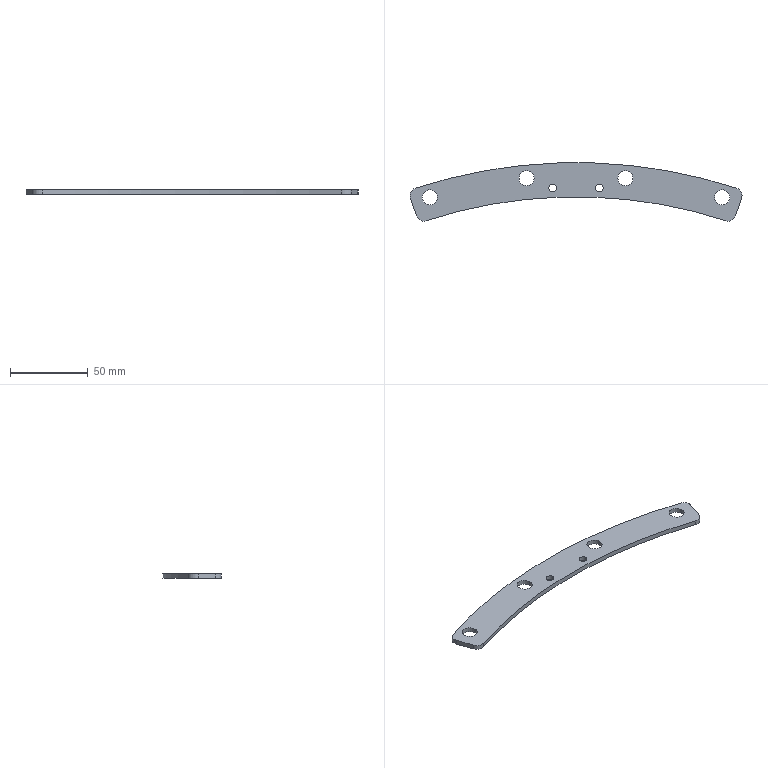Part | 1 solid | 23 faces | box 213.441 x 37.571 x 3 mm | volume 12982 mm3 | cylinder 19 | plane 4 | commonest cylinder face diameters 9.7 x8 10 x5 5 x4 620 x1 664 x1
STEP:
#1=CARTESIAN_POINT('',(-17.5,315.7,-3.));
#2=VERTEX_POINT('',#1);
#3=CARTESIAN_POINT('',(-12.5,315.7,-3.));
#4=VERTEX_POINT('',#3);
#5=CARTESIAN_POINT('',(-15.,315.7,-3.));
#6=DIRECTION('',(0.,0.,1.));
#7=DIRECTION('',(1.,0.,0.));
#8=AXIS2_PLACEMENT_3D('',#5,#6,#7);
#9=CIRCLE('',#8,2.5);
#10=EDGE_CURVE('',#2,#4,#9,.T.);
#11=ORIENTED_EDGE('',*,*,#10,.F.);
#12=CARTESIAN_POINT('',(-17.5,315.7,0.));
#13=VERTEX_POINT('',#12);
#14=CARTESIAN_POINT('',(-17.5,315.7,0.));
#15=DIRECTION('',(0.,0.,1.));
#16=VECTOR('',#15,1000.);
#17=LINE('',#14,#16);
#18=EDGE_CURVE('',#2,#13,#17,.T.);
#19=ORIENTED_EDGE('',*,*,#18,.T.);
#20=CARTESIAN_POINT('',(-12.5,315.7,0.));
#21=VERTEX_POINT('',#20);
#22=CARTESIAN_POINT('',(-15.,315.7,0.));
#23=DIRECTION('',(0.,0.,1.));
#24=DIRECTION('',(1.,0.,0.));
#25=AXIS2_PLACEMENT_3D('',#22,#23,#24);
#26=CIRCLE('',#25,2.5);
#27=EDGE_CURVE('',#13,#21,#26,.T.);
#28=ORIENTED_EDGE('',*,*,#27,.T.);
#29=CARTESIAN_POINT('',(-12.5,315.7,0.));
#30=DIRECTION('',(0.,0.,1.));
#31=VECTOR('',#30,1000.);
#32=LINE('',#29,#31);
#33=EDGE_CURVE('',#4,#21,#32,.T.);
#34=ORIENTED_EDGE('',*,*,#33,.F.);
#35=EDGE_LOOP('',(#11,#19,#28,#34));
#36=FACE_OUTER_BOUND('',#35,.T.);
#37=CARTESIAN_POINT('',(-15.,315.7,0.));
#38=DIRECTION('',(0.,0.,1.));
#39=DIRECTION('',(1.,0.,0.));
#40=AXIS2_PLACEMENT_3D('',#37,#38,#39);
#41=CYLINDRICAL_SURFACE('',#40,2.5);
#42=ADVANCED_FACE('',(#36),#41,.F.);
#43=CARTESIAN_POINT('',(12.5,315.7,-3.));
#44=VERTEX_POINT('',#43);
#45=CARTESIAN_POINT('',(17.5,315.7,-3.));
#46=VERTEX_POINT('',#45);
#47=CARTESIAN_POINT('',(15.,315.7,-3.));
#48=DIRECTION('',(0.,0.,1.));
#49=DIRECTION('',(1.,0.,0.));
#50=AXIS2_PLACEMENT_3D('',#47,#48,#49);
#51=CIRCLE('',#50,2.5);
#52=EDGE_CURVE('',#44,#46,#51,.T.);
#53=ORIENTED_EDGE('',*,*,#52,.F.);
#54=CARTESIAN_POINT('',(12.5,315.7,0.));
#55=VERTEX_POINT('',#54);
#56=CARTESIAN_POINT('',(12.5,315.7,0.));
#57=DIRECTION('',(0.,0.,1.));
#58=VECTOR('',#57,1000.);
#59=LINE('',#56,#58);
#60=EDGE_CURVE('',#44,#55,#59,.T.);
#61=ORIENTED_EDGE('',*,*,#60,.T.);
#62=CARTESIAN_POINT('',(17.5,315.7,0.));
#63=VERTEX_POINT('',#62);
#64=CARTESIAN_POINT('',(15.,315.7,0.));
#65=DIRECTION('',(0.,0.,1.));
#66=DIRECTION('',(1.,0.,0.));
#67=AXIS2_PLACEMENT_3D('',#64,#65,#66);
#68=CIRCLE('',#67,2.5);
#69=EDGE_CURVE('',#55,#63,#68,.T.);
#70=ORIENTED_EDGE('',*,*,#69,.T.);
#71=CARTESIAN_POINT('',(17.5,315.7,0.));
#72=DIRECTION('',(0.,0.,1.));
#73=VECTOR('',#72,1000.);
#74=LINE('',#71,#73);
#75=EDGE_CURVE('',#46,#63,#74,.T.);
#76=ORIENTED_EDGE('',*,*,#75,.F.);
#77=EDGE_LOOP('',(#53,#61,#70,#76));
#78=FACE_OUTER_BOUND('',#77,.T.);
#79=CARTESIAN_POINT('',(15.,315.7,0.));
#80=DIRECTION('',(0.,0.,1.));
#81=DIRECTION('',(1.,0.,0.));
#82=AXIS2_PLACEMENT_3D('',#79,#80,#81);
#83=CYLINDRICAL_SURFACE('',#82,2.5);
#84=ADVANCED_FACE('',(#78),#83,.F.);
#85=CARTESIAN_POINT('',(-89.15,309.625,-3.));
#86=VERTEX_POINT('',#85);
#87=CARTESIAN_POINT('',(-98.85,309.625,-3.));
#88=VERTEX_POINT('',#87);
#89=CARTESIAN_POINT('',(-94.,309.625,-3.));
#90=DIRECTION('',(0.,0.,-1.));
#91=DIRECTION('',(-1.,0.,0.));
#92=AXIS2_PLACEMENT_3D('',#89,#90,#91);
#93=CIRCLE('',#92,4.85);
#94=EDGE_CURVE('',#86,#88,#93,.T.);
#95=ORIENTED_EDGE('',*,*,#94,.T.);
#96=CARTESIAN_POINT('',(-98.85,309.625,0.));
#97=VERTEX_POINT('',#96);
#98=CARTESIAN_POINT('',(-98.85,309.625,-10.));
#99=DIRECTION('',(0.,0.,1.));
#100=VECTOR('',#99,1000.);
#101=LINE('',#98,#100);
#102=EDGE_CURVE('',#88,#97,#101,.T.);
#103=ORIENTED_EDGE('',*,*,#102,.T.);
#104=CARTESIAN_POINT('',(-89.15,309.625,0.));
#105=VERTEX_POINT('',#104);
#106=CARTESIAN_POINT('',(-94.,309.625,0.));
#107=DIRECTION('',(0.,0.,1.));
#108=DIRECTION('',(-1.,0.,0.));
#109=AXIS2_PLACEMENT_3D('',#106,#107,#108);
#110=CIRCLE('',#109,4.85);
#111=EDGE_CURVE('',#97,#105,#110,.T.);
#112=ORIENTED_EDGE('',*,*,#111,.T.);
#113=CARTESIAN_POINT('',(-89.15,309.625,-10.));
#114=DIRECTION('',(0.,0.,1.));
#115=VECTOR('',#114,1000.);
#116=LINE('',#113,#115);
#117=EDGE_CURVE('',#86,#105,#116,.T.);
#118=ORIENTED_EDGE('',*,*,#117,.F.);
#119=EDGE_LOOP('',(#95,#103,#112,#118));
#120=FACE_OUTER_BOUND('',#119,.T.);
#121=CARTESIAN_POINT('',(-94.,309.625,-10.));
#122=DIRECTION('',(0.,0.,1.));
#123=DIRECTION('',(1.,0.,0.));
#124=AXIS2_PLACEMENT_3D('',#121,#122,#123);
#125=CYLINDRICAL_SURFACE('',#124,4.85);
#126=ADVANCED_FACE('',(#120),#125,.F.);
#127=CARTESIAN_POINT('',(98.85,309.625,-3.));
#128=VERTEX_POINT('',#127);
#129=CARTESIAN_POINT('',(89.15,309.625,-3.));
#130=VERTEX_POINT('',#129);
#131=CARTESIAN_POINT('',(94.,309.625,-3.));
#132=DIRECTION('',(0.,0.,-1.));
#133=DIRECTION('',(-1.,0.,0.));
#134=AXIS2_PLACEMENT_3D('',#131,#132,#133);
#135=CIRCLE('',#134,4.85);
#136=EDGE_CURVE('',#128,#130,#135,.T.);
#137=ORIENTED_EDGE('',*,*,#136,.T.);
#138=CARTESIAN_POINT('',(89.15,309.625,0.));
#139=VERTEX_POINT('',#138);
#140=CARTESIAN_POINT('',(89.15,309.625,-10.));
#141=DIRECTION('',(0.,0.,1.));
#142=VECTOR('',#141,1000.);
#143=LINE('',#140,#142);
#144=EDGE_CURVE('',#130,#139,#143,.T.);
#145=ORIENTED_EDGE('',*,*,#144,.T.);
#146=CARTESIAN_POINT('',(98.85,309.625,0.));
#147=VERTEX_POINT('',#146);
#148=CARTESIAN_POINT('',(94.,309.625,0.));
#149=DIRECTION('',(0.,0.,1.));
#150=DIRECTION('',(1.,0.,0.));
#151=AXIS2_PLACEMENT_3D('',#148,#149,#150);
#152=CIRCLE('',#151,4.85);
#153=EDGE_CURVE('',#139,#147,#152,.T.);
#154=ORIENTED_EDGE('',*,*,#153,.T.);
#155=CARTESIAN_POINT('',(98.85,309.625,-10.));
#156=DIRECTION('',(0.,0.,1.));
#157=VECTOR('',#156,1000.);
#158=LINE('',#155,#157);
#159=EDGE_CURVE('',#128,#147,#158,.T.);
#160=ORIENTED_EDGE('',*,*,#159,.F.);
#161=EDGE_LOOP('',(#137,#145,#154,#160));
#162=FACE_OUTER_BOUND('',#161,.T.);
#163=CARTESIAN_POINT('',(94.,309.625,-10.));
#164=DIRECTION('',(0.,0.,1.));
#165=DIRECTION('',(1.,0.,0.));
#166=AXIS2_PLACEMENT_3D('',#163,#164,#165);
#167=CYLINDRICAL_SURFACE('',#166,4.85);
#168=ADVANCED_FACE('',(#162),#167,.F.);
#169=CARTESIAN_POINT('',(36.6,322.001,-3.));
#170=VERTEX_POINT('',#169);
#171=CARTESIAN_POINT('',(26.9,322.001,-3.));
#172=VERTEX_POINT('',#171);
#173=CARTESIAN_POINT('',(31.75,322.001,-3.));
#174=DIRECTION('',(0.,0.,-1.));
#175=DIRECTION('',(-1.,0.,0.));
#176=AXIS2_PLACEMENT_3D('',#173,#174,#175);
#177=CIRCLE('',#176,4.85);
#178=EDGE_CURVE('',#170,#172,#177,.T.);
#179=ORIENTED_EDGE('',*,*,#178,.T.);
#180=CARTESIAN_POINT('',(26.9,322.001,0.));
#181=VERTEX_POINT('',#180);
#182=CARTESIAN_POINT('',(26.9,322.001,-10.));
#183=DIRECTION('',(0.,0.,1.));
#184=VECTOR('',#183,1000.);
#185=LINE('',#182,#184);
#186=EDGE_CURVE('',#172,#181,#185,.T.);
#187=ORIENTED_EDGE('',*,*,#186,.T.);
#188=CARTESIAN_POINT('',(36.6,322.001,0.));
#189=VERTEX_POINT('',#188);
#190=CARTESIAN_POINT('',(31.75,322.001,0.));
#191=DIRECTION('',(0.,0.,1.));
#192=DIRECTION('',(1.,0.,0.));
#193=AXIS2_PLACEMENT_3D('',#190,#191,#192);
#194=CIRCLE('',#193,4.85);
#195=EDGE_CURVE('',#181,#189,#194,.T.);
#196=ORIENTED_EDGE('',*,*,#195,.T.);
#197=CARTESIAN_POINT('',(36.6,322.001,-10.));
#198=DIRECTION('',(0.,0.,1.));
#199=VECTOR('',#198,1000.);
#200=LINE('',#197,#199);
#201=EDGE_CURVE('',#170,#189,#200,.T.);
#202=ORIENTED_EDGE('',*,*,#201,.F.);
#203=EDGE_LOOP('',(#179,#187,#196,#202));
#204=FACE_OUTER_BOUND('',#203,.T.);
#205=CARTESIAN_POINT('',(31.75,322.001,-10.));
#206=DIRECTION('',(0.,0.,1.));
#207=DIRECTION('',(1.,0.,0.));
#208=AXIS2_PLACEMENT_3D('',#205,#206,#207);
#209=CYLINDRICAL_SURFACE('',#208,4.85);
#210=ADVANCED_FACE('',(#204),#209,.F.);
#211=CARTESIAN_POINT('',(-26.9,322.001,-3.));
#212=VERTEX_POINT('',#211);
#213=CARTESIAN_POINT('',(-36.6,322.001,-3.));
#214=VERTEX_POINT('',#213);
#215=CARTESIAN_POINT('',(-31.75,322.001,-3.));
#216=DIRECTION('',(0.,0.,-1.));
#217=DIRECTION('',(-1.,0.,0.));
#218=AXIS2_PLACEMENT_3D('',#215,#216,#217);
#219=CIRCLE('',#218,4.85);
#220=EDGE_CURVE('',#212,#214,#219,.T.);
#221=ORIENTED_EDGE('',*,*,#220,.T.);
#222=CARTESIAN_POINT('',(-36.6,322.001,0.));
#223=VERTEX_POINT('',#222);
#224=CARTESIAN_POINT('',(-36.6,322.001,-10.));
#225=DIRECTION('',(0.,0.,1.));
#226=VECTOR('',#225,1000.);
#227=LINE('',#224,#226);
#228=EDGE_CURVE('',#214,#223,#227,.T.);
#229=ORIENTED_EDGE('',*,*,#228,.T.);
#230=CARTESIAN_POINT('',(-26.9,322.001,0.));
#231=VERTEX_POINT('',#230);
#232=CARTESIAN_POINT('',(-31.75,322.001,0.));
#233=DIRECTION('',(0.,0.,1.));
#234=DIRECTION('',(-1.,0.,0.));
#235=AXIS2_PLACEMENT_3D('',#232,#233,#234);
#236=CIRCLE('',#235,4.85);
#237=EDGE_CURVE('',#223,#231,#236,.T.);
#238=ORIENTED_EDGE('',*,*,#237,.T.);
#239=CARTESIAN_POINT('',(-26.9,322.001,-10.));
#240=DIRECTION('',(0.,0.,1.));
#241=VECTOR('',#240,1000.);
#242=LINE('',#239,#241);
#243=EDGE_CURVE('',#212,#231,#242,.T.);
#244=ORIENTED_EDGE('',*,*,#243,.F.);
#245=EDGE_LOOP('',(#221,#229,#238,#244));
#246=FACE_OUTER_BOUND('',#245,.T.);
#247=CARTESIAN_POINT('',(-31.75,322.001,-10.));
#248=DIRECTION('',(0.,0.,1.));
#249=DIRECTION('',(1.,0.,0.));
#250=AXIS2_PLACEMENT_3D('',#247,#248,#249);
#251=CYLINDRICAL_SURFACE('',#250,4.85);
#252=ADVANCED_FACE('',(#246),#251,.F.);
#253=CARTESIAN_POINT('',(106.721,310.776,-3.));
#254=VERTEX_POINT('',#253);
#255=CARTESIAN_POINT('',(106.448,309.148,-3.));
#256=VERTEX_POINT('',#255);
#257=CARTESIAN_POINT('',(101.721,310.776,-3.));
#258=DIRECTION('',(0.,0.,-1.));
#259=DIRECTION('',(-1.,0.,0.));
#260=AXIS2_PLACEMENT_3D('',#257,#258,#259);
#261=CIRCLE('',#260,5.);
#262=EDGE_CURVE('',#254,#256,#261,.T.);
#263=ORIENTED_EDGE('',*,*,#262,.F.);
#264=CARTESIAN_POINT('',(106.721,310.776,0.));
#265=VERTEX_POINT('',#264);
#266=CARTESIAN_POINT('',(106.721,310.776,-3.));
#267=DIRECTION('',(0.,0.,1.));
#268=VECTOR('',#267,1000.);
#269=LINE('',#266,#268);
#270=EDGE_CURVE('',#254,#265,#269,.T.);
#271=ORIENTED_EDGE('',*,*,#270,.T.);
#272=CARTESIAN_POINT('',(106.448,309.148,0.));
#273=VERTEX_POINT('',#272);
#274=CARTESIAN_POINT('',(101.721,310.776,0.));
#275=DIRECTION('',(0.,0.,1.));
#276=DIRECTION('',(-1.,0.,0.));
#277=AXIS2_PLACEMENT_3D('',#274,#275,#276);
#278=CIRCLE('',#277,5.);
#279=EDGE_CURVE('',#273,#265,#278,.T.);
#280=ORIENTED_EDGE('',*,*,#279,.F.);
#281=CARTESIAN_POINT('',(106.448,309.148,-3.));
#282=DIRECTION('',(0.,0.,1.));
#283=VECTOR('',#282,1000.);
#284=LINE('',#281,#283);
#285=EDGE_CURVE('',#256,#273,#284,.T.);
#286=ORIENTED_EDGE('',*,*,#285,.F.);
#287=EDGE_LOOP('',(#263,#271,#280,#286));
#288=FACE_OUTER_BOUND('',#287,.T.);
#289=CARTESIAN_POINT('',(101.721,310.776,-3.));
#290=DIRECTION('',(0.,0.,1.));
#291=DIRECTION('',(1.,0.,0.));
#292=AXIS2_PLACEMENT_3D('',#289,#290,#291);
#293=CYLINDRICAL_SURFACE('',#292,5.);
#294=ADVANCED_FACE('',(#288),#293,.T.);
#295=CARTESIAN_POINT('',(-96.261,294.676,-3.));
#296=VERTEX_POINT('',#295);
#297=CARTESIAN_POINT('',(96.261,294.676,-3.));
#298=VERTEX_POINT('',#297);
#299=CARTESIAN_POINT('',(0.,0.,-3.));
#300=DIRECTION('',(0.,0.,-1.));
#301=DIRECTION('',(-1.,0.,0.));
#302=AXIS2_PLACEMENT_3D('',#299,#300,#301);
#303=CIRCLE('',#302,310.);
#304=EDGE_CURVE('',#296,#298,#303,.T.);
#305=ORIENTED_EDGE('',*,*,#304,.T.);
#306=CARTESIAN_POINT('',(96.261,294.676,0.));
#307=VERTEX_POINT('',#306);
#308=CARTESIAN_POINT('',(96.261,294.676,-3.));
#309=DIRECTION('',(0.,0.,1.));
#310=VECTOR('',#309,1000.);
#311=LINE('',#308,#310);
#312=EDGE_CURVE('',#298,#307,#311,.T.);
#313=ORIENTED_EDGE('',*,*,#312,.T.);
#314=CARTESIAN_POINT('',(-96.261,294.676,0.));
#315=VERTEX_POINT('',#314);
#316=CARTESIAN_POINT('',(0.,0.,0.));
#317=DIRECTION('',(0.,0.,-1.));
#318=DIRECTION('',(-1.,0.,0.));
#319=AXIS2_PLACEMENT_3D('',#316,#317,#318);
#320=CIRCLE('',#319,310.);
#321=EDGE_CURVE('',#315,#307,#320,.T.);
#322=ORIENTED_EDGE('',*,*,#321,.F.);
#323=CARTESIAN_POINT('',(-96.261,294.676,-3.));
#324=DIRECTION('',(0.,0.,-1.));
#325=VECTOR('',#324,1000.);
#326=LINE('',#323,#325);
#327=EDGE_CURVE('',#315,#296,#326,.T.);
#328=ORIENTED_EDGE('',*,*,#327,.T.);
#329=EDGE_LOOP('',(#305,#313,#322,#328));
#330=FACE_OUTER_BOUND('',#329,.T.);
#331=CARTESIAN_POINT('',(0.,0.,-3.));
#332=DIRECTION('',(0.,0.,1.));
#333=DIRECTION('',(1.,0.,0.));
#334=AXIS2_PLACEMENT_3D('',#331,#332,#333);
#335=CYLINDRICAL_SURFACE('',#334,310.);
#336=ADVANCED_FACE('',(#330),#335,.F.);
#337=CARTESIAN_POINT('',(-106.448,309.148,-3.));
#338=VERTEX_POINT('',#337);
#339=CARTESIAN_POINT('',(-102.541,297.801,-3.));
#340=VERTEX_POINT('',#339);
#341=CARTESIAN_POINT('',(-100.926,293.111,-3.));
#342=DIRECTION('',(0.3256,-0.9455,0.));
#343=VECTOR('',#342,1000.);
#344=LINE('',#341,#343);
#345=EDGE_CURVE('',#338,#340,#344,.T.);
#346=ORIENTED_EDGE('',*,*,#345,.T.);
#347=CARTESIAN_POINT('',(-102.541,297.801,0.));
#348=VERTEX_POINT('',#347);
#349=CARTESIAN_POINT('',(-102.541,297.801,-3.));
#350=DIRECTION('',(0.,0.,1.));
#351=VECTOR('',#350,1000.);
#352=LINE('',#349,#351);
#353=EDGE_CURVE('',#340,#348,#352,.T.);
#354=ORIENTED_EDGE('',*,*,#353,.T.);
#355=CARTESIAN_POINT('',(-106.448,309.148,0.));
#356=VERTEX_POINT('',#355);
#357=CARTESIAN_POINT('',(-100.926,293.111,0.));
#358=DIRECTION('',(0.3256,-0.9455,0.));
#359=VECTOR('',#358,1000.);
#360=LINE('',#357,#359);
#361=EDGE_CURVE('',#356,#348,#360,.T.);
#362=ORIENTED_EDGE('',*,*,#361,.F.);
#363=CARTESIAN_POINT('',(-106.448,309.148,-3.));
#364=DIRECTION('',(0.,0.,-1.));
#365=VECTOR('',#364,1000.);
#366=LINE('',#363,#365);
#367=EDGE_CURVE('',#356,#338,#366,.T.);
#368=ORIENTED_EDGE('',*,*,#367,.T.);
#369=EDGE_LOOP('',(#346,#354,#362,#368));
#370=FACE_OUTER_BOUND('',#369,.T.);
#371=CARTESIAN_POINT('',(-100.926,293.111,-3.));
#372=DIRECTION('',(-0.9455,-0.3256,0.));
#373=DIRECTION('',(0.3256,-0.9455,0.));
#374=AXIS2_PLACEMENT_3D('',#371,#372,#373);
#375=PLANE('',#374);
#376=ADVANCED_FACE('',(#370),#375,.T.);
#377=CARTESIAN_POINT('',(103.276,315.528,0.));
#378=VERTEX_POINT('',#377);
#379=CARTESIAN_POINT('',(-103.276,315.528,0.));
#380=VERTEX_POINT('',#379);
#381=CARTESIAN_POINT('',(0.,0.,0.));
#382=DIRECTION('',(0.,0.,1.));
#383=DIRECTION('',(-1.,0.,0.));
#384=AXIS2_PLACEMENT_3D('',#381,#382,#383);
#385=CIRCLE('',#384,332.);
#386=EDGE_CURVE('',#378,#380,#385,.T.);
#387=ORIENTED_EDGE('',*,*,#386,.F.);
#388=CARTESIAN_POINT('',(103.276,315.528,-3.));
#389=VERTEX_POINT('',#388);
#390=CARTESIAN_POINT('',(103.276,315.528,-3.));
#391=DIRECTION('',(0.,0.,-1.));
#392=VECTOR('',#391,1000.);
#393=LINE('',#390,#392);
#394=EDGE_CURVE('',#378,#389,#393,.T.);
#395=ORIENTED_EDGE('',*,*,#394,.T.);
#396=CARTESIAN_POINT('',(-103.276,315.528,-3.));
#397=VERTEX_POINT('',#396);
#398=CARTESIAN_POINT('',(0.,0.,-3.));
#399=DIRECTION('',(0.,0.,1.));
#400=DIRECTION('',(-1.,0.,0.));
#401=AXIS2_PLACEMENT_3D('',#398,#399,#400);
#402=CIRCLE('',#401,332.);
#403=EDGE_CURVE('',#389,#397,#402,.T.);
#404=ORIENTED_EDGE('',*,*,#403,.T.);
#405=CARTESIAN_POINT('',(-103.276,315.528,-3.));
#406=DIRECTION('',(0.,0.,1.));
#407=VECTOR('',#406,1000.);
#408=LINE('',#405,#407);
#409=EDGE_CURVE('',#397,#380,#408,.T.);
#410=ORIENTED_EDGE('',*,*,#409,.T.);
#411=EDGE_LOOP('',(#387,#395,#404,#410));
#412=FACE_OUTER_BOUND('',#411,.T.);
#413=CARTESIAN_POINT('',(0.,0.,-3.));
#414=DIRECTION('',(0.,0.,1.));
#415=DIRECTION('',(1.,0.,0.));
#416=AXIS2_PLACEMENT_3D('',#413,#414,#415);
#417=CYLINDRICAL_SURFACE('',#416,332.);
#418=ADVANCED_FACE('',(#412),#417,.T.);
#419=CARTESIAN_POINT('',(102.541,297.801,0.));
#420=VERTEX_POINT('',#419);
#421=CARTESIAN_POINT('',(100.926,293.111,0.));
#422=DIRECTION('',(0.3256,0.9455,0.));
#423=VECTOR('',#422,1000.);
#424=LINE('',#421,#423);
#425=EDGE_CURVE('',#420,#273,#424,.T.);
#426=ORIENTED_EDGE('',*,*,#425,.F.);
#427=CARTESIAN_POINT('',(102.541,297.801,-3.));
#428=VERTEX_POINT('',#427);
#429=CARTESIAN_POINT('',(102.541,297.801,-3.));
#430=DIRECTION('',(0.,0.,-1.));
#431=VECTOR('',#430,1000.);
#432=LINE('',#429,#431);
#433=EDGE_CURVE('',#420,#428,#432,.T.);
#434=ORIENTED_EDGE('',*,*,#433,.T.);
#435=CARTESIAN_POINT('',(100.926,293.111,-3.));
#436=DIRECTION('',(0.3256,0.9455,0.));
#437=VECTOR('',#436,1000.);
#438=LINE('',#435,#437);
#439=EDGE_CURVE('',#428,#256,#438,.T.);
#440=ORIENTED_EDGE('',*,*,#439,.T.);
#441=ORIENTED_EDGE('',*,*,#285,.T.);
#442=EDGE_LOOP('',(#426,#434,#440,#441));
#443=FACE_OUTER_BOUND('',#442,.T.);
#444=CARTESIAN_POINT('',(100.926,293.111,-3.));
#445=DIRECTION('',(0.9455,-0.3256,0.));
#446=DIRECTION('',(0.3256,0.9455,0.));
#447=AXIS2_PLACEMENT_3D('',#444,#445,#446);
#448=PLANE('',#447);
#449=ADVANCED_FACE('',(#443),#448,.T.);
#450=CARTESIAN_POINT('',(-15.,315.7,-3.));
#451=DIRECTION('',(0.,0.,1.));
#452=DIRECTION('',(1.,0.,0.));
#453=AXIS2_PLACEMENT_3D('',#450,#451,#452);
#454=CIRCLE('',#453,2.5);
#455=EDGE_CURVE('',#4,#2,#454,.T.);
#456=ORIENTED_EDGE('',*,*,#455,.T.);
#457=ORIENTED_EDGE('',*,*,#10,.T.);
#458=EDGE_LOOP('',(#456,#457));
#459=FACE_BOUND('',#458,.T.);
#460=CARTESIAN_POINT('',(15.,315.7,-3.));
#461=DIRECTION('',(0.,0.,1.));
#462=DIRECTION('',(1.,0.,0.));
#463=AXIS2_PLACEMENT_3D('',#460,#461,#462);
#464=CIRCLE('',#463,2.5);
#465=EDGE_CURVE('',#46,#44,#464,.T.);
#466=ORIENTED_EDGE('',*,*,#465,.T.);
#467=ORIENTED_EDGE('',*,*,#52,.T.);
#468=EDGE_LOOP('',(#466,#467));
#469=FACE_BOUND('',#468,.T.);
#470=ORIENTED_EDGE('',*,*,#94,.F.);
#471=CARTESIAN_POINT('',(-94.,309.625,-3.));
#472=DIRECTION('',(0.,0.,-1.));
#473=DIRECTION('',(-1.,0.,0.));
#474=AXIS2_PLACEMENT_3D('',#471,#472,#473);
#475=CIRCLE('',#474,4.85);
#476=EDGE_CURVE('',#88,#86,#475,.T.);
#477=ORIENTED_EDGE('',*,*,#476,.F.);
#478=EDGE_LOOP('',(#470,#477));
#479=FACE_BOUND('',#478,.T.);
#480=ORIENTED_EDGE('',*,*,#136,.F.);
#481=CARTESIAN_POINT('',(94.,309.625,-3.));
#482=DIRECTION('',(0.,0.,-1.));
#483=DIRECTION('',(-1.,0.,0.));
#484=AXIS2_PLACEMENT_3D('',#481,#482,#483);
#485=CIRCLE('',#484,4.85);
#486=EDGE_CURVE('',#130,#128,#485,.T.);
#487=ORIENTED_EDGE('',*,*,#486,.F.);
#488=EDGE_LOOP('',(#480,#487));
#489=FACE_BOUND('',#488,.T.);
#490=ORIENTED_EDGE('',*,*,#178,.F.);
#491=CARTESIAN_POINT('',(31.75,322.001,-3.));
#492=DIRECTION('',(0.,0.,-1.));
#493=DIRECTION('',(-1.,0.,0.));
#494=AXIS2_PLACEMENT_3D('',#491,#492,#493);
#495=CIRCLE('',#494,4.85);
#496=EDGE_CURVE('',#172,#170,#495,.T.);
#497=ORIENTED_EDGE('',*,*,#496,.F.);
#498=EDGE_LOOP('',(#490,#497));
#499=FACE_BOUND('',#498,.T.);
#500=ORIENTED_EDGE('',*,*,#220,.F.);
#501=CARTESIAN_POINT('',(-31.75,322.001,-3.));
#502=DIRECTION('',(0.,0.,-1.));
#503=DIRECTION('',(-1.,0.,0.));
#504=AXIS2_PLACEMENT_3D('',#501,#502,#503);
#505=CIRCLE('',#504,4.85);
#506=EDGE_CURVE('',#214,#212,#505,.T.);
#507=ORIENTED_EDGE('',*,*,#506,.F.);
#508=EDGE_LOOP('',(#500,#507));
#509=FACE_BOUND('',#508,.T.);
#510=ORIENTED_EDGE('',*,*,#439,.F.);
#511=CARTESIAN_POINT('',(97.813,299.429,-3.));
#512=DIRECTION('',(0.,0.,-1.));
#513=DIRECTION('',(-1.,0.,0.));
#514=AXIS2_PLACEMENT_3D('',#511,#512,#513);
#515=CIRCLE('',#514,5.);
#516=EDGE_CURVE('',#428,#298,#515,.T.);
#517=ORIENTED_EDGE('',*,*,#516,.T.);
#518=ORIENTED_EDGE('',*,*,#304,.F.);
#519=CARTESIAN_POINT('',(-97.813,299.429,-3.));
#520=DIRECTION('',(0.,0.,-1.));
#521=DIRECTION('',(-1.,0.,0.));
#522=AXIS2_PLACEMENT_3D('',#519,#520,#521);
#523=CIRCLE('',#522,5.);
#524=EDGE_CURVE('',#296,#340,#523,.T.);
#525=ORIENTED_EDGE('',*,*,#524,.T.);
#526=ORIENTED_EDGE('',*,*,#345,.F.);
#527=CARTESIAN_POINT('',(-101.721,310.776,-3.));
#528=DIRECTION('',(0.,0.,-1.));
#529=DIRECTION('',(-1.,0.,0.));
#530=AXIS2_PLACEMENT_3D('',#527,#528,#529);
#531=CIRCLE('',#530,5.);
#532=EDGE_CURVE('',#338,#397,#531,.T.);
#533=ORIENTED_EDGE('',*,*,#532,.T.);
#534=ORIENTED_EDGE('',*,*,#403,.F.);
#535=CARTESIAN_POINT('',(101.721,310.776,-3.));
#536=DIRECTION('',(0.,0.,-1.));
#537=DIRECTION('',(-1.,0.,0.));
#538=AXIS2_PLACEMENT_3D('',#535,#536,#537);
#539=CIRCLE('',#538,5.);
#540=EDGE_CURVE('',#389,#254,#539,.T.);
#541=ORIENTED_EDGE('',*,*,#540,.T.);
#542=ORIENTED_EDGE('',*,*,#262,.T.);
#543=EDGE_LOOP('',(#510,#517,#518,#525,#526,#533,#534,#541,#542));
#544=FACE_OUTER_BOUND('',#543,.T.);
#545=CARTESIAN_POINT('',(0.,0.,-3.));
#546=DIRECTION('',(0.,0.,-1.));
#547=DIRECTION('',(-1.,0.,0.));
#548=AXIS2_PLACEMENT_3D('',#545,#546,#547);
#549=PLANE('',#548);
#550=ADVANCED_FACE('',(#459,#469,#479,#489,#499,#509,#544),#549,.T.);
#551=CARTESIAN_POINT('',(-15.,315.7,0.));
#552=DIRECTION('',(0.,0.,1.));
#553=DIRECTION('',(1.,0.,0.));
#554=AXIS2_PLACEMENT_3D('',#551,#552,#553);
#555=CIRCLE('',#554,2.5);
#556=EDGE_CURVE('',#21,#13,#555,.T.);
#557=ORIENTED_EDGE('',*,*,#556,.F.);
#558=ORIENTED_EDGE('',*,*,#27,.F.);
#559=EDGE_LOOP('',(#557,#558));
#560=FACE_BOUND('',#559,.T.);
#561=CARTESIAN_POINT('',(15.,315.7,0.));
#562=DIRECTION('',(0.,0.,1.));
#563=DIRECTION('',(1.,0.,0.));
#564=AXIS2_PLACEMENT_3D('',#561,#562,#563);
#565=CIRCLE('',#564,2.5);
#566=EDGE_CURVE('',#63,#55,#565,.T.);
#567=ORIENTED_EDGE('',*,*,#566,.F.);
#568=ORIENTED_EDGE('',*,*,#69,.F.);
#569=EDGE_LOOP('',(#567,#568));
#570=FACE_BOUND('',#569,.T.);
#571=CARTESIAN_POINT('',(-94.,309.625,0.));
#572=DIRECTION('',(0.,0.,1.));
#573=DIRECTION('',(-1.,0.,0.));
#574=AXIS2_PLACEMENT_3D('',#571,#572,#573);
#575=CIRCLE('',#574,4.85);
#576=EDGE_CURVE('',#105,#97,#575,.T.);
#577=ORIENTED_EDGE('',*,*,#576,.F.);
#578=ORIENTED_EDGE('',*,*,#111,.F.);
#579=EDGE_LOOP('',(#577,#578));
#580=FACE_BOUND('',#579,.T.);
#581=CARTESIAN_POINT('',(94.,309.625,0.));
#582=DIRECTION('',(0.,0.,1.));
#583=DIRECTION('',(1.,0.,0.));
#584=AXIS2_PLACEMENT_3D('',#581,#582,#583);
#585=CIRCLE('',#584,4.85);
#586=EDGE_CURVE('',#147,#139,#585,.T.);
#587=ORIENTED_EDGE('',*,*,#586,.F.);
#588=ORIENTED_EDGE('',*,*,#153,.F.);
#589=EDGE_LOOP('',(#587,#588));
#590=FACE_BOUND('',#589,.T.);
#591=CARTESIAN_POINT('',(31.75,322.001,0.));
#592=DIRECTION('',(0.,0.,1.));
#593=DIRECTION('',(1.,0.,0.));
#594=AXIS2_PLACEMENT_3D('',#591,#592,#593);
#595=CIRCLE('',#594,4.85);
#596=EDGE_CURVE('',#189,#181,#595,.T.);
#597=ORIENTED_EDGE('',*,*,#596,.F.);
#598=ORIENTED_EDGE('',*,*,#195,.F.);
#599=EDGE_LOOP('',(#597,#598));
#600=FACE_BOUND('',#599,.T.);
#601=CARTESIAN_POINT('',(-31.75,322.001,0.));
#602=DIRECTION('',(0.,0.,1.));
#603=DIRECTION('',(-1.,0.,0.));
#604=AXIS2_PLACEMENT_3D('',#601,#602,#603);
#605=CIRCLE('',#604,4.85);
#606=EDGE_CURVE('',#231,#223,#605,.T.);
#607=ORIENTED_EDGE('',*,*,#606,.F.);
#608=ORIENTED_EDGE('',*,*,#237,.F.);
#609=EDGE_LOOP('',(#607,#608));
#610=FACE_BOUND('',#609,.T.);
#611=ORIENTED_EDGE('',*,*,#321,.T.);
#612=CARTESIAN_POINT('',(97.813,299.429,0.));
#613=DIRECTION('',(0.,0.,1.));
#614=DIRECTION('',(-1.,0.,0.));
#615=AXIS2_PLACEMENT_3D('',#612,#613,#614);
#616=CIRCLE('',#615,5.);
#617=EDGE_CURVE('',#307,#420,#616,.T.);
#618=ORIENTED_EDGE('',*,*,#617,.T.);
#619=ORIENTED_EDGE('',*,*,#425,.T.);
#620=ORIENTED_EDGE('',*,*,#279,.T.);
#621=CARTESIAN_POINT('',(101.721,310.776,0.));
#622=DIRECTION('',(0.,0.,1.));
#623=DIRECTION('',(-1.,0.,0.));
#624=AXIS2_PLACEMENT_3D('',#621,#622,#623);
#625=CIRCLE('',#624,5.);
#626=EDGE_CURVE('',#265,#378,#625,.T.);
#627=ORIENTED_EDGE('',*,*,#626,.T.);
#628=ORIENTED_EDGE('',*,*,#386,.T.);
#629=CARTESIAN_POINT('',(-101.721,310.776,0.));
#630=DIRECTION('',(0.,0.,1.));
#631=DIRECTION('',(-1.,0.,0.));
#632=AXIS2_PLACEMENT_3D('',#629,#630,#631);
#633=CIRCLE('',#632,5.);
#634=EDGE_CURVE('',#380,#356,#633,.T.);
#635=ORIENTED_EDGE('',*,*,#634,.T.);
#636=ORIENTED_EDGE('',*,*,#361,.T.);
#637=CARTESIAN_POINT('',(-97.813,299.429,0.));
#638=DIRECTION('',(0.,0.,1.));
#639=DIRECTION('',(-1.,0.,0.));
#640=AXIS2_PLACEMENT_3D('',#637,#638,#639);
#641=CIRCLE('',#640,5.);
#642=EDGE_CURVE('',#348,#315,#641,.T.);
#643=ORIENTED_EDGE('',*,*,#642,.T.);
#644=EDGE_LOOP('',(#611,#618,#619,#620,#627,#628,#635,#636,#643));
#645=FACE_OUTER_BOUND('',#644,.T.);
#646=CARTESIAN_POINT('',(0.,0.,0.));
#647=DIRECTION('',(0.,0.,-1.));
#648=DIRECTION('',(-1.,0.,0.));
#649=AXIS2_PLACEMENT_3D('',#646,#647,#648);
#650=PLANE('',#649);
#651=ADVANCED_FACE('',(#560,#570,#580,#590,#600,#610,#645),#650,.F.);
#652=ORIENTED_EDGE('',*,*,#516,.F.);
#653=ORIENTED_EDGE('',*,*,#433,.F.);
#654=ORIENTED_EDGE('',*,*,#617,.F.);
#655=ORIENTED_EDGE('',*,*,#312,.F.);
#656=EDGE_LOOP('',(#652,#653,#654,#655));
#657=FACE_OUTER_BOUND('',#656,.T.);
#658=CARTESIAN_POINT('',(97.813,299.429,-3.));
#659=DIRECTION('',(0.,0.,1.));
#660=DIRECTION('',(1.,0.,0.));
#661=AXIS2_PLACEMENT_3D('',#658,#659,#660);
#662=CYLINDRICAL_SURFACE('',#661,5.);
#663=ADVANCED_FACE('',(#657),#662,.T.);
#664=ORIENTED_EDGE('',*,*,#270,.F.);
#665=ORIENTED_EDGE('',*,*,#540,.F.);
#666=ORIENTED_EDGE('',*,*,#394,.F.);
#667=ORIENTED_EDGE('',*,*,#626,.F.);
#668=EDGE_LOOP('',(#664,#665,#666,#667));
#669=FACE_OUTER_BOUND('',#668,.T.);
#670=CARTESIAN_POINT('',(101.721,310.776,-3.));
#671=DIRECTION('',(0.,0.,1.));
#672=DIRECTION('',(1.,0.,0.));
#673=AXIS2_PLACEMENT_3D('',#670,#671,#672);
#674=CYLINDRICAL_SURFACE('',#673,5.);
#675=ADVANCED_FACE('',(#669),#674,.T.);
#676=ORIENTED_EDGE('',*,*,#524,.F.);
#677=ORIENTED_EDGE('',*,*,#327,.F.);
#678=ORIENTED_EDGE('',*,*,#642,.F.);
#679=ORIENTED_EDGE('',*,*,#353,.F.);
#680=EDGE_LOOP('',(#676,#677,#678,#679));
#681=FACE_OUTER_BOUND('',#680,.T.);
#682=CARTESIAN_POINT('',(-97.813,299.429,-3.));
#683=DIRECTION('',(0.,0.,1.));
#684=DIRECTION('',(1.,0.,0.));
#685=AXIS2_PLACEMENT_3D('',#682,#683,#684);
#686=CYLINDRICAL_SURFACE('',#685,5.);
#687=ADVANCED_FACE('',(#681),#686,.T.);
#688=ORIENTED_EDGE('',*,*,#532,.F.);
#689=ORIENTED_EDGE('',*,*,#367,.F.);
#690=ORIENTED_EDGE('',*,*,#634,.F.);
#691=ORIENTED_EDGE('',*,*,#409,.F.);
#692=EDGE_LOOP('',(#688,#689,#690,#691));
#693=FACE_OUTER_BOUND('',#692,.T.);
#694=CARTESIAN_POINT('',(-101.721,310.776,-3.));
#695=DIRECTION('',(0.,0.,1.));
#696=DIRECTION('',(1.,0.,0.));
#697=AXIS2_PLACEMENT_3D('',#694,#695,#696);
#698=CYLINDRICAL_SURFACE('',#697,5.);
#699=ADVANCED_FACE('',(#693),#698,.T.);
#700=ORIENTED_EDGE('',*,*,#228,.F.);
#701=ORIENTED_EDGE('',*,*,#506,.T.);
#702=ORIENTED_EDGE('',*,*,#243,.T.);
#703=ORIENTED_EDGE('',*,*,#606,.T.);
#704=EDGE_LOOP('',(#700,#701,#702,#703));
#705=FACE_OUTER_BOUND('',#704,.T.);
#706=CARTESIAN_POINT('',(-31.75,322.001,-10.));
#707=DIRECTION('',(0.,0.,1.));
#708=DIRECTION('',(1.,0.,0.));
#709=AXIS2_PLACEMENT_3D('',#706,#707,#708);
#710=CYLINDRICAL_SURFACE('',#709,4.85);
#711=ADVANCED_FACE('',(#705),#710,.F.);
#712=ORIENTED_EDGE('',*,*,#186,.F.);
#713=ORIENTED_EDGE('',*,*,#496,.T.);
#714=ORIENTED_EDGE('',*,*,#201,.T.);
#715=ORIENTED_EDGE('',*,*,#596,.T.);
#716=EDGE_LOOP('',(#712,#713,#714,#715));
#717=FACE_OUTER_BOUND('',#716,.T.);
#718=CARTESIAN_POINT('',(31.75,322.001,-10.));
#719=DIRECTION('',(0.,0.,1.));
#720=DIRECTION('',(1.,0.,0.));
#721=AXIS2_PLACEMENT_3D('',#718,#719,#720);
#722=CYLINDRICAL_SURFACE('',#721,4.85);
#723=ADVANCED_FACE('',(#717),#722,.F.);
#724=ORIENTED_EDGE('',*,*,#144,.F.);
#725=ORIENTED_EDGE('',*,*,#486,.T.);
#726=ORIENTED_EDGE('',*,*,#159,.T.);
#727=ORIENTED_EDGE('',*,*,#586,.T.);
#728=EDGE_LOOP('',(#724,#725,#726,#727));
#729=FACE_OUTER_BOUND('',#728,.T.);
#730=CARTESIAN_POINT('',(94.,309.625,-10.));
#731=DIRECTION('',(0.,0.,1.));
#732=DIRECTION('',(1.,0.,0.));
#733=AXIS2_PLACEMENT_3D('',#730,#731,#732);
#734=CYLINDRICAL_SURFACE('',#733,4.85);
#735=ADVANCED_FACE('',(#729),#734,.F.);
#736=ORIENTED_EDGE('',*,*,#102,.F.);
#737=ORIENTED_EDGE('',*,*,#476,.T.);
#738=ORIENTED_EDGE('',*,*,#117,.T.);
#739=ORIENTED_EDGE('',*,*,#576,.T.);
#740=EDGE_LOOP('',(#736,#737,#738,#739));
#741=FACE_OUTER_BOUND('',#740,.T.);
#742=CARTESIAN_POINT('',(-94.,309.625,-10.));
#743=DIRECTION('',(0.,0.,1.));
#744=DIRECTION('',(1.,0.,0.));
#745=AXIS2_PLACEMENT_3D('',#742,#743,#744);
#746=CYLINDRICAL_SURFACE('',#745,4.85);
#747=ADVANCED_FACE('',(#741),#746,.F.);
#748=ORIENTED_EDGE('',*,*,#60,.F.);
#749=ORIENTED_EDGE('',*,*,#465,.F.);
#750=ORIENTED_EDGE('',*,*,#75,.T.);
#751=ORIENTED_EDGE('',*,*,#566,.T.);
#752=EDGE_LOOP('',(#748,#749,#750,#751));
#753=FACE_OUTER_BOUND('',#752,.T.);
#754=CARTESIAN_POINT('',(15.,315.7,0.));
#755=DIRECTION('',(0.,0.,1.));
#756=DIRECTION('',(1.,0.,0.));
#757=AXIS2_PLACEMENT_3D('',#754,#755,#756);
#758=CYLINDRICAL_SURFACE('',#757,2.5);
#759=ADVANCED_FACE('',(#753),#758,.F.);
#760=ORIENTED_EDGE('',*,*,#18,.F.);
#761=ORIENTED_EDGE('',*,*,#455,.F.);
#762=ORIENTED_EDGE('',*,*,#33,.T.);
#763=ORIENTED_EDGE('',*,*,#556,.T.);
#764=EDGE_LOOP('',(#760,#761,#762,#763));
#765=FACE_OUTER_BOUND('',#764,.T.);
#766=CARTESIAN_POINT('',(-15.,315.7,0.));
#767=DIRECTION('',(0.,0.,1.));
#768=DIRECTION('',(1.,0.,0.));
#769=AXIS2_PLACEMENT_3D('',#766,#767,#768);
#770=CYLINDRICAL_SURFACE('',#769,2.5);
#771=ADVANCED_FACE('',(#765),#770,.F.);
#772=CLOSED_SHELL('',(#42,#84,#126,#168,#210,#252,#294,#336,#376,#418,#449,#550,#651,#663,#675,#687,#699,#711,#723,#735,#747,#759,#771));
#773=MANIFOLD_SOLID_BREP('',#772);
#774=CARTESIAN_POINT('',(0.,0.,0.));
#775=DIRECTION('',(0.,0.,1.));
#776=DIRECTION('',(1.,0.,0.));
#777=AXIS2_PLACEMENT_3D('',#774,#775,#776);
#778=(LENGTH_UNIT()NAMED_UNIT(*)SI_UNIT(.MILLI.,.METRE.));
#779=UNCERTAINTY_MEASURE_WITH_UNIT(LENGTH_MEASURE(0.00001),#778,'','');
#780=(NAMED_UNIT(*)PLANE_ANGLE_UNIT()SI_UNIT($,.RADIAN.));
#781=(NAMED_UNIT(*)SI_UNIT($,.STERADIAN.)SOLID_ANGLE_UNIT());
#782=(GEOMETRIC_REPRESENTATION_CONTEXT(3)GLOBAL_UNCERTAINTY_ASSIGNED_CONTEXT((#779))GLOBAL_UNIT_ASSIGNED_CONTEXT((#778,#780,#781))REPRESENTATION_CONTEXT('',''));
#783=ADVANCED_BREP_SHAPE_REPRESENTATION('',(#773,#777),#782);